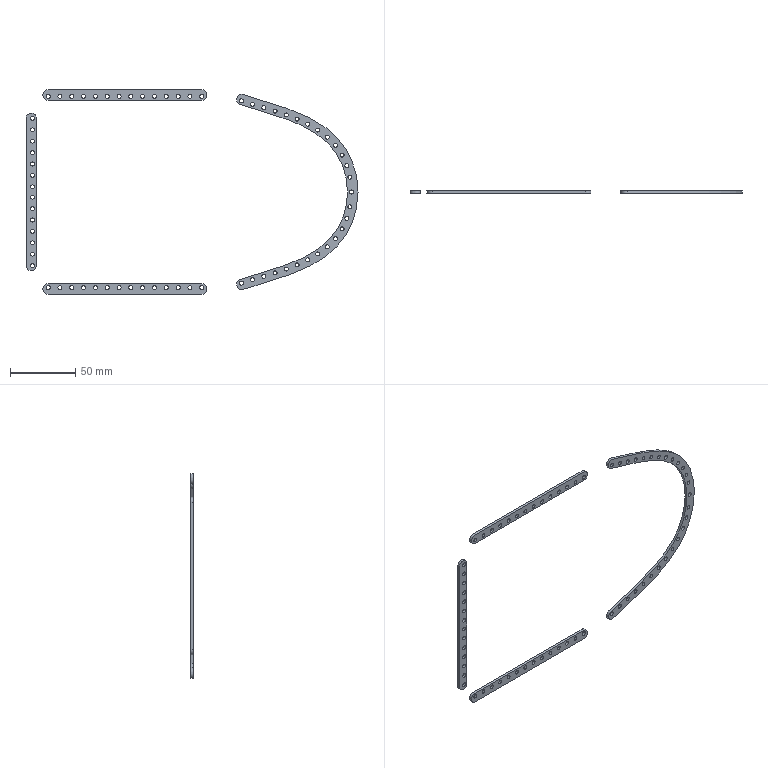Part | SolidWorks | features Extrusion 1 | 4 solids | 166 faces | box 255.002 x 2 x 157 mm | volume 8812 mm3 | cylinder 148 | plane 14 | spline 4 | commonest cylinder face diameters 3.1 x138 8 x10